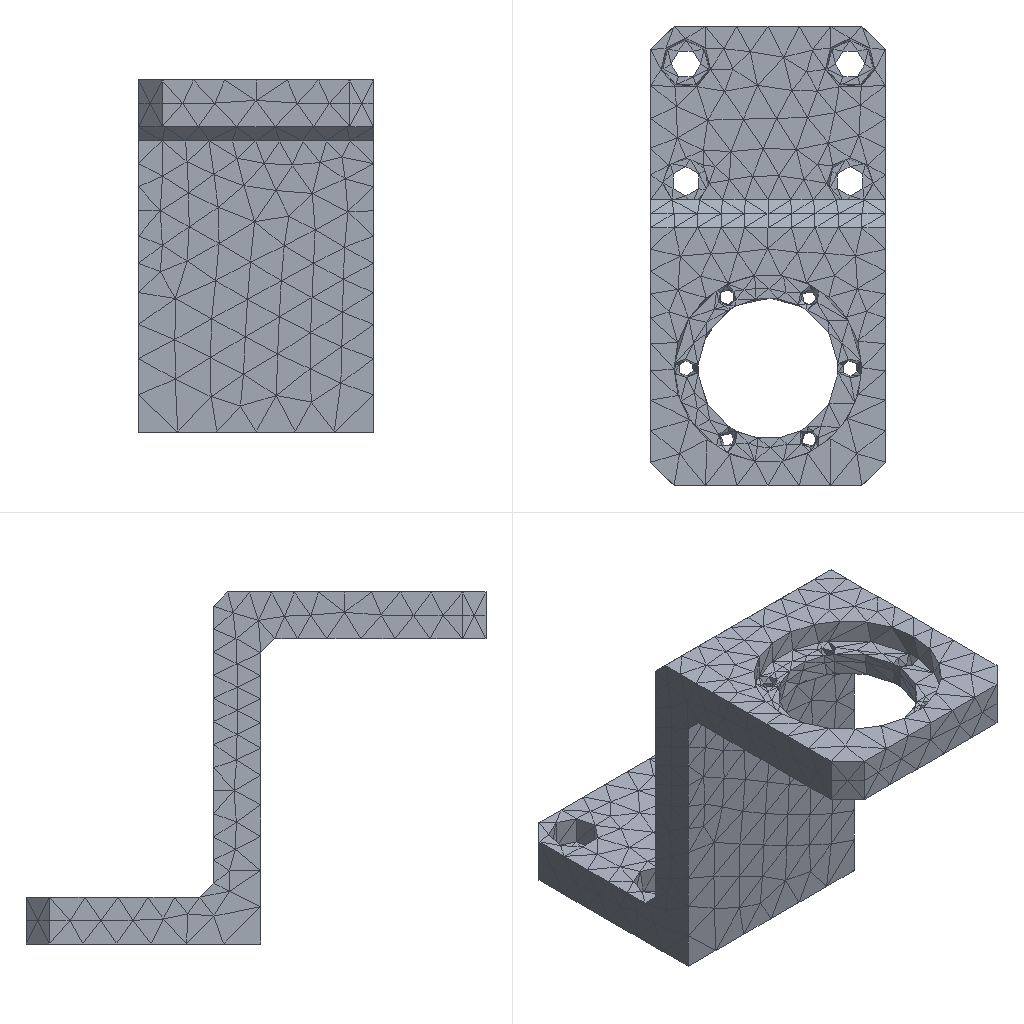Simulation study | nx simcenter
Set-up summary:
category,name,step,type,value,unit,region
solver,nx_nastran (Simcenter)
units,not stated in the deck,,not stated
analysis,deck,,static,static
analysis,solution,,SOL,101
load_step,SUBCASE 1,1,SUBCASE,SPC=1 LOAD=2
load_step,requested,,,1
mesh,nodes,,,5294
mesh,elements,,,2569
element_type,CTETRA,,solid,2569
load,nodal force total,,FX,0.0,model units
load,nodal force total,,FY,0.0,model units
load,nodal force total,,FZ,-3000000.03,model units
load,load commands in deck,,count,147
bc,support commands in deck,,count,451
analysis,NX solution 0,,Structural,Linear Statics - Single Constraint
check,setup vs results,,match,every grid point's frame and coordinates and every element id; grid points of CTETRA elements
Nastran input file, long lists of numbers shortened:
$*$$$$$$$$$$$$$$$$$$$$$$$$$$$$$$$$$$$$$$$$$$$$$$$$$$$$$$$$$$$$$$$$$
$*
$*                    NX v10.0.0.24 TRANSLATOR
$*                    FOR NX NASTRAN VERSION 10.0
$ (33 more lines like these left out)
ASSIGN OUTPUT2='142_sim1-solution_1.op2' UNIT=12
$*
$*$$$$$$$$$$$$$$$$$$$$$$$$$$$$$$$$$$$
$*
$* EXECUTIVE CONTROL
$*
$*$$$$$$$$$$$$$$$$$$$$$$$$$$$$$$$$$$$
$*
ID,NASTRAN,142_sim1-solution_1
SOL 101
CEND
$*
$*$$$$$$$$$$$$$$$$$$$$$$$$$$$$$$$$$$$
$*
$* CASE CONTROL
$*
$*$$$$$$$$$$$$$$$$$$$$$$$$$$$$$$$$$$$
$*
TITLE = Solution 1
ECHO = NONE
SPC = 1
OUTPUT
BCRESULTS(TRACTION,FORCE,PLOT) = ALL
DISPLACEMENT(PLOT) = ALL
ESE(PLOT) = ALL
FORCE(PLOT,CORNER) = ALL
OLOAD(PLOT) = ALL
SPCFORCES(PLOT) = ALL
STRAIN(PLOT,FIBER,CORNER) = ALL
STRESS(PLOT,CORNER) = ALL
$*  NX Step: Subcase - Static Loads 1
SUBCASE 1
LABEL = Subcase - Static Loads 1
LOAD = 2
$*
$*$$$$$$$$$$$$$$$$$$$$$$$$$$$$$$$$$$$
$*
$* BULK DATA
$*
$*$$$$$$$$$$$$$$$$$$$$$$$$$$$$$$$$$$$
$*
BEGIN BULK
$*
$* PARAM CARDS
$*
PARAM      K6ROT100.0000
PARAM     OIBULK     YES
PARAM    OMACHPR     YES
PARAM       POST      -2
PARAM    POSTEXT     YES
PARAM    UNITSYS   MN-MM
$*
$* GRID CARDS
$*
GRID*               5196               0-2.500000000E+01-4.300000000E+01+
*       6.5000000000E+01               0
GRID*               5197               0-2.500000000E+01-4.300000000E+01+
*       7.5000000000E+01               0
$ (10584 more lines like these left out)
$*
$* ELEMENT CARDS
$*
$*  NX Mesh Collector: Solid(1)
$*  NX Mesh: 3d_mesh(1)
CTETRA         1       1    1988       1    1993    1987      48      49+
+           2058    2049      50    2059
CTETRA         2       1       2    1987    1995    1993      51    2068+
+             52      53    2059    2069
$ (5134 more lines like these left out)
$*
$* PROPERTY CARDS
$*
$*  NX Property: PSOLID1
PSOLID         1       1       0                           SMECH
$*
$* MATERIAL CARDS
$*
$*  NX Material: Aluminum_2014
MAT1           17.3119+7        0.3300002.7940-62.1355-5
MATT1          1       1               2               3
TABLEM1        1                                                        +
+        20.00007.3119+7 21.11007.3119+7 23.89007.3119+7 37.78007.3119+7+
+        51.67007.3119+7 65.56007.2429+7 79.44007.2429+7 93.33007.1739+7+
+       107.22007.1049+7121.11007.0359+7135.00006.9670+7148.89006.8980+7+
+       162.78006.8290+7176.67006.6910+7190.56006.6221+7204.44006.4841+7+
+       218.33006.3461+7232.22006.1392+7246.11006.0012+7260.00005.8633+7+
+       273.89005.7253+7287.78005.5184+7301.67005.3804+7315.56005.1735+7+
+       329.44004.9665+7343.33004.7596+7357.22004.6216+7371.11004.4147+7+
+           ENDT
TABLEM1        2                                                        +
+        20.00000.330000 21.11000.330000    ENDT
TABLEM1        3                                                        +
+        20.00002.1600-5 93.33002.2500-5107.22002.2662-5121.11002.2824-5+
+       135.00002.2968-5148.89002.3130-5162.78002.3274-5176.67002.3418-5+
+       190.56002.3544-5204.44002.3688-5218.33002.3814-5232.22002.3958-5+
+       246.11002.4066-5260.00002.4192-5273.89002.4300-5287.78002.4408-5+
+       301.67002.4498-5315.56002.4606-5329.44002.4696-5343.33002.4786-5+
+       357.22002.4876-5371.11002.4984-5385.00002.5110-5398.89002.5254-5+
+       412.78002.5398-5426.67002.5560-5    ENDT
$*
$* LOAD AND CONSTRAINT CARDS
$*
$*  NX Load and Constraint: Fixed(1)
SPC            1    3182  123456  0.0000
SPC            1    3183  123456  0.0000
SPC            1    3184  123456  0.0000
SPC            1    3185  123456  0.0000
$ (447 more lines like these left out)
$*  NX Load and Constraint: Force(1)
FORCE          2    2897       043325.90  0.0000  0.0000-1.00000
FORCE          2    2898       019963.36  0.0000  0.0000-1.00000
FORCE          2    2899       056890.22  0.0000  0.0000-1.00000
FORCE          2    2900       042669.17  0.0000  0.0000-1.00000
$ (143 more lines like these left out)
ENDDATA ba1229b9
Results summary:
result,analysis,,,static
result,last_loadstep,,,1
result,primary field,,,displacements
result,reaction total,,FX,0.01385,model units
result,reaction total,,FY,0.6959,model units
result,reaction total,,FZ,3000000.25,model units
result,NX solution 0,,loadcases,1,mm